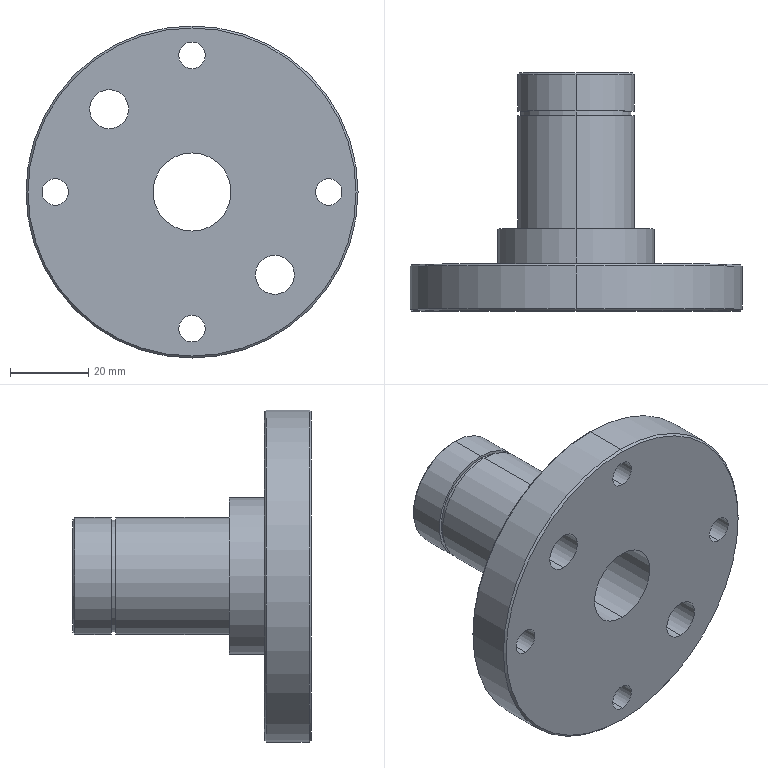Part | SolidWorks | features HoleWzd 2, Chamfer 1, ICE 1, RevCut 1, Revolution 1 | 1 solid | 38 faces | box 85 x 61 x 85 mm | volume 84723 mm3 | cylinder 24 | cone 8 | plane 6 | commonest cylinder face diameters 6.8 x8 10 x4 30 x4 20 x2 28.6 x2 40 x2
STEP:
#1=CARTESIAN_POINT('',(0.,60.5,-10.));
#2=VERTEX_POINT('',#1);
#3=CARTESIAN_POINT('',(0.,60.5,10.));
#4=VERTEX_POINT('',#3);
#5=CARTESIAN_POINT('',(0.,60.5,0.));
#6=DIRECTION('',(0.,1.,0.));
#7=DIRECTION('',(0.,0.,1.));
#8=AXIS2_PLACEMENT_3D('',#5,#6,#7);
#9=CIRCLE('',#8,10.);
#10=EDGE_CURVE('',#2,#4,#9,.T.);
#11=ORIENTED_EDGE('',*,*,#10,.F.);
#12=CARTESIAN_POINT('',(0.,61.,-10.5));
#13=VERTEX_POINT('',#12);
#14=CARTESIAN_POINT('',(0.,60.5,-10.));
#15=DIRECTION('',(0.,0.7071,-0.7071));
#16=VECTOR('',#15,1000.);
#17=LINE('',#14,#16);
#18=EDGE_CURVE('',#2,#13,#17,.T.);
#19=ORIENTED_EDGE('',*,*,#18,.T.);
#20=CARTESIAN_POINT('',(0.,61.,10.5));
#21=VERTEX_POINT('',#20);
#22=CARTESIAN_POINT('',(0.,61.,0.));
#23=DIRECTION('',(0.,-1.,0.));
#24=DIRECTION('',(0.,0.,1.));
#25=AXIS2_PLACEMENT_3D('',#22,#23,#24);
#26=CIRCLE('',#25,10.5);
#27=EDGE_CURVE('',#21,#13,#26,.T.);
#28=ORIENTED_EDGE('',*,*,#27,.F.);
#29=CARTESIAN_POINT('',(0.,60.5,10.));
#30=DIRECTION('',(0.,0.7071,0.7071));
#31=VECTOR('',#30,1000.);
#32=LINE('',#29,#31);
#33=EDGE_CURVE('',#4,#21,#32,.T.);
#34=ORIENTED_EDGE('',*,*,#33,.F.);
#35=EDGE_LOOP('',(#11,#19,#28,#34));
#36=FACE_OUTER_BOUND('',#35,.T.);
#37=CARTESIAN_POINT('',(0.,60.5,0.));
#38=DIRECTION('',(0.,1.,0.));
#39=DIRECTION('',(0.,0.,1.));
#40=AXIS2_PLACEMENT_3D('',#37,#38,#39);
#41=CONICAL_SURFACE('',#40,10.,0.7854);
#42=ADVANCED_FACE('',(#36),#41,.F.);
#43=CARTESIAN_POINT('',(0.,61.,14.5));
#44=VERTEX_POINT('',#43);
#45=CARTESIAN_POINT('',(0.,61.,-14.5));
#46=VERTEX_POINT('',#45);
#47=CARTESIAN_POINT('',(0.,61.,0.));
#48=DIRECTION('',(0.,1.,0.));
#49=DIRECTION('',(0.,0.,1.));
#50=AXIS2_PLACEMENT_3D('',#47,#48,#49);
#51=CIRCLE('',#50,14.5);
#52=EDGE_CURVE('',#44,#46,#51,.T.);
#53=ORIENTED_EDGE('',*,*,#52,.F.);
#54=CARTESIAN_POINT('',(0.,60.5,15.));
#55=VERTEX_POINT('',#54);
#56=CARTESIAN_POINT('',(0.,60.5,15.));
#57=DIRECTION('',(0.,-0.7071,0.7071));
#58=VECTOR('',#57,1000.);
#59=LINE('',#56,#58);
#60=EDGE_CURVE('',#44,#55,#59,.T.);
#61=ORIENTED_EDGE('',*,*,#60,.T.);
#62=CARTESIAN_POINT('',(0.,60.5,-15.));
#63=VERTEX_POINT('',#62);
#64=CARTESIAN_POINT('',(0.,60.5,0.));
#65=DIRECTION('',(0.,-1.,0.));
#66=DIRECTION('',(0.,0.,1.));
#67=AXIS2_PLACEMENT_3D('',#64,#65,#66);
#68=CIRCLE('',#67,15.);
#69=EDGE_CURVE('',#63,#55,#68,.T.);
#70=ORIENTED_EDGE('',*,*,#69,.F.);
#71=CARTESIAN_POINT('',(0.,60.5,-15.));
#72=DIRECTION('',(0.,-0.7071,-0.7071));
#73=VECTOR('',#72,1000.);
#74=LINE('',#71,#73);
#75=EDGE_CURVE('',#46,#63,#74,.T.);
#76=ORIENTED_EDGE('',*,*,#75,.F.);
#77=EDGE_LOOP('',(#53,#61,#70,#76));
#78=FACE_OUTER_BOUND('',#77,.T.);
#79=CARTESIAN_POINT('',(0.,60.5,0.));
#80=DIRECTION('',(0.,-1.,0.));
#81=DIRECTION('',(0.,0.,-1.));
#82=AXIS2_PLACEMENT_3D('',#79,#80,#81);
#83=CONICAL_SURFACE('',#82,15.,0.7854);
#84=ADVANCED_FACE('',(#78),#83,.T.);
#85=CARTESIAN_POINT('',(0.,12.,42.));
#86=VERTEX_POINT('',#85);
#87=CARTESIAN_POINT('',(0.,12.,-42.));
#88=VERTEX_POINT('',#87);
#89=CARTESIAN_POINT('',(0.,12.,0.));
#90=DIRECTION('',(0.,1.,0.));
#91=DIRECTION('',(0.,0.,1.));
#92=AXIS2_PLACEMENT_3D('',#89,#90,#91);
#93=CIRCLE('',#92,42.);
#94=EDGE_CURVE('',#86,#88,#93,.T.);
#95=ORIENTED_EDGE('',*,*,#94,.F.);
#96=CARTESIAN_POINT('',(0.,11.5,42.5));
#97=VERTEX_POINT('',#96);
#98=CARTESIAN_POINT('',(0.,11.5,42.5));
#99=DIRECTION('',(0.,-0.7071,0.7071));
#100=VECTOR('',#99,1000.);
#101=LINE('',#98,#100);
#102=EDGE_CURVE('',#86,#97,#101,.T.);
#103=ORIENTED_EDGE('',*,*,#102,.T.);
#104=CARTESIAN_POINT('',(0.,11.5,-42.5));
#105=VERTEX_POINT('',#104);
#106=CARTESIAN_POINT('',(0.,11.5,0.));
#107=DIRECTION('',(0.,-1.,0.));
#108=DIRECTION('',(0.,0.,1.));
#109=AXIS2_PLACEMENT_3D('',#106,#107,#108);
#110=CIRCLE('',#109,42.5);
#111=EDGE_CURVE('',#105,#97,#110,.T.);
#112=ORIENTED_EDGE('',*,*,#111,.F.);
#113=CARTESIAN_POINT('',(0.,11.5,-42.5));
#114=DIRECTION('',(0.,-0.7071,-0.7071));
#115=VECTOR('',#114,1000.);
#116=LINE('',#113,#115);
#117=EDGE_CURVE('',#88,#105,#116,.T.);
#118=ORIENTED_EDGE('',*,*,#117,.F.);
#119=EDGE_LOOP('',(#95,#103,#112,#118));
#120=FACE_OUTER_BOUND('',#119,.T.);
#121=CARTESIAN_POINT('',(0.,11.5,0.));
#122=DIRECTION('',(0.,-1.,0.));
#123=DIRECTION('',(0.,0.,-1.));
#124=AXIS2_PLACEMENT_3D('',#121,#122,#123);
#125=CONICAL_SURFACE('',#124,42.5,0.7854);
#126=ADVANCED_FACE('',(#120),#125,.T.);
#127=CARTESIAN_POINT('',(0.,0.,-42.));
#128=VERTEX_POINT('',#127);
#129=CARTESIAN_POINT('',(0.,0.,42.));
#130=VERTEX_POINT('',#129);
#131=CARTESIAN_POINT('',(0.,0.,0.));
#132=DIRECTION('',(0.,-1.,0.));
#133=DIRECTION('',(0.,0.,-1.));
#134=AXIS2_PLACEMENT_3D('',#131,#132,#133);
#135=CIRCLE('',#134,42.);
#136=EDGE_CURVE('',#128,#130,#135,.T.);
#137=ORIENTED_EDGE('',*,*,#136,.F.);
#138=CARTESIAN_POINT('',(0.,0.5,-42.5));
#139=VERTEX_POINT('',#138);
#140=CARTESIAN_POINT('',(0.,0.,-42.));
#141=DIRECTION('',(0.,0.7071,-0.7071));
#142=VECTOR('',#141,1000.);
#143=LINE('',#140,#142);
#144=EDGE_CURVE('',#128,#139,#143,.T.);
#145=ORIENTED_EDGE('',*,*,#144,.T.);
#146=CARTESIAN_POINT('',(0.,0.5,42.5));
#147=VERTEX_POINT('',#146);
#148=CARTESIAN_POINT('',(0.,0.5,0.));
#149=DIRECTION('',(0.,1.,0.));
#150=DIRECTION('',(0.,0.,-1.));
#151=AXIS2_PLACEMENT_3D('',#148,#149,#150);
#152=CIRCLE('',#151,42.5);
#153=EDGE_CURVE('',#147,#139,#152,.T.);
#154=ORIENTED_EDGE('',*,*,#153,.F.);
#155=CARTESIAN_POINT('',(0.,0.,42.));
#156=DIRECTION('',(0.,0.7071,0.7071));
#157=VECTOR('',#156,1000.);
#158=LINE('',#155,#157);
#159=EDGE_CURVE('',#130,#147,#158,.T.);
#160=ORIENTED_EDGE('',*,*,#159,.F.);
#161=EDGE_LOOP('',(#137,#145,#154,#160));
#162=FACE_OUTER_BOUND('',#161,.T.);
#163=CARTESIAN_POINT('',(0.,0.,0.));
#164=DIRECTION('',(0.,1.,0.));
#165=DIRECTION('',(0.,0.,1.));
#166=AXIS2_PLACEMENT_3D('',#163,#164,#165);
#167=CONICAL_SURFACE('',#166,42.,0.7854);
#168=ADVANCED_FACE('',(#162),#167,.T.);
#169=CARTESIAN_POINT('',(-21.213,0.,16.213));
#170=VERTEX_POINT('',#169);
#171=CARTESIAN_POINT('',(-21.213,0.,26.213));
#172=VERTEX_POINT('',#171);
#173=CARTESIAN_POINT('',(-21.213,0.,21.213));
#174=DIRECTION('',(0.,1.,0.));
#175=DIRECTION('',(0.,0.,1.));
#176=AXIS2_PLACEMENT_3D('',#173,#174,#175);
#177=CIRCLE('',#176,5.);
#178=EDGE_CURVE('',#170,#172,#177,.T.);
#179=ORIENTED_EDGE('',*,*,#178,.F.);
#180=CARTESIAN_POINT('',(-21.213,12.,16.213));
#181=VERTEX_POINT('',#180);
#182=CARTESIAN_POINT('',(-21.213,12.,16.213));
#183=DIRECTION('',(0.,1.,0.));
#184=VECTOR('',#183,1000.);
#185=LINE('',#182,#184);
#186=EDGE_CURVE('',#170,#181,#185,.T.);
#187=ORIENTED_EDGE('',*,*,#186,.T.);
#188=CARTESIAN_POINT('',(-21.213,12.,26.213));
#189=VERTEX_POINT('',#188);
#190=CARTESIAN_POINT('',(-21.213,12.,21.213));
#191=DIRECTION('',(0.,1.,0.));
#192=DIRECTION('',(0.,0.,1.));
#193=AXIS2_PLACEMENT_3D('',#190,#191,#192);
#194=CIRCLE('',#193,5.);
#195=EDGE_CURVE('',#181,#189,#194,.T.);
#196=ORIENTED_EDGE('',*,*,#195,.T.);
#197=CARTESIAN_POINT('',(-21.213,12.,26.213));
#198=DIRECTION('',(0.,1.,0.));
#199=VECTOR('',#198,1000.);
#200=LINE('',#197,#199);
#201=EDGE_CURVE('',#172,#189,#200,.T.);
#202=ORIENTED_EDGE('',*,*,#201,.F.);
#203=EDGE_LOOP('',(#179,#187,#196,#202));
#204=FACE_OUTER_BOUND('',#203,.T.);
#205=CARTESIAN_POINT('',(-21.213,12.,21.213));
#206=DIRECTION('',(0.,1.,0.));
#207=DIRECTION('',(0.,0.,1.));
#208=AXIS2_PLACEMENT_3D('',#205,#206,#207);
#209=CYLINDRICAL_SURFACE('',#208,5.);
#210=ADVANCED_FACE('',(#204),#209,.F.);
#211=CARTESIAN_POINT('',(21.213,0.,-26.213));
#212=VERTEX_POINT('',#211);
#213=CARTESIAN_POINT('',(21.213,0.,-16.213));
#214=VERTEX_POINT('',#213);
#215=CARTESIAN_POINT('',(21.213,0.,-21.213));
#216=DIRECTION('',(0.,1.,0.));
#217=DIRECTION('',(0.,0.,1.));
#218=AXIS2_PLACEMENT_3D('',#215,#216,#217);
#219=CIRCLE('',#218,5.);
#220=EDGE_CURVE('',#212,#214,#219,.T.);
#221=ORIENTED_EDGE('',*,*,#220,.F.);
#222=CARTESIAN_POINT('',(21.213,12.,-26.213));
#223=VERTEX_POINT('',#222);
#224=CARTESIAN_POINT('',(21.213,12.,-26.213));
#225=DIRECTION('',(0.,1.,0.));
#226=VECTOR('',#225,1000.);
#227=LINE('',#224,#226);
#228=EDGE_CURVE('',#212,#223,#227,.T.);
#229=ORIENTED_EDGE('',*,*,#228,.T.);
#230=CARTESIAN_POINT('',(21.213,12.,-16.213));
#231=VERTEX_POINT('',#230);
#232=CARTESIAN_POINT('',(21.213,12.,-21.213));
#233=DIRECTION('',(0.,1.,0.));
#234=DIRECTION('',(0.,0.,1.));
#235=AXIS2_PLACEMENT_3D('',#232,#233,#234);
#236=CIRCLE('',#235,5.);
#237=EDGE_CURVE('',#223,#231,#236,.T.);
#238=ORIENTED_EDGE('',*,*,#237,.T.);
#239=CARTESIAN_POINT('',(21.213,12.,-16.213));
#240=DIRECTION('',(0.,1.,0.));
#241=VECTOR('',#240,1000.);
#242=LINE('',#239,#241);
#243=EDGE_CURVE('',#214,#231,#242,.T.);
#244=ORIENTED_EDGE('',*,*,#243,.F.);
#245=EDGE_LOOP('',(#221,#229,#238,#244));
#246=FACE_OUTER_BOUND('',#245,.T.);
#247=CARTESIAN_POINT('',(21.213,12.,-21.213));
#248=DIRECTION('',(0.,1.,0.));
#249=DIRECTION('',(0.,0.,1.));
#250=AXIS2_PLACEMENT_3D('',#247,#248,#249);
#251=CYLINDRICAL_SURFACE('',#250,5.);
#252=ADVANCED_FACE('',(#246),#251,.F.);
#253=CARTESIAN_POINT('',(35.,0.,-3.4));
#254=VERTEX_POINT('',#253);
#255=CARTESIAN_POINT('',(35.,0.,3.4));
#256=VERTEX_POINT('',#255);
#257=CARTESIAN_POINT('',(35.,0.,0.));
#258=DIRECTION('',(0.,1.,0.));
#259=DIRECTION('',(0.,0.,1.));
#260=AXIS2_PLACEMENT_3D('',#257,#258,#259);
#261=CIRCLE('',#260,3.4);
#262=EDGE_CURVE('',#254,#256,#261,.T.);
#263=ORIENTED_EDGE('',*,*,#262,.F.);
#264=CARTESIAN_POINT('',(35.,12.,-3.4));
#265=VERTEX_POINT('',#264);
#266=CARTESIAN_POINT('',(35.,12.,-3.4));
#267=DIRECTION('',(0.,1.,0.));
#268=VECTOR('',#267,1000.);
#269=LINE('',#266,#268);
#270=EDGE_CURVE('',#254,#265,#269,.T.);
#271=ORIENTED_EDGE('',*,*,#270,.T.);
#272=CARTESIAN_POINT('',(35.,12.,3.4));
#273=VERTEX_POINT('',#272);
#274=CARTESIAN_POINT('',(35.,12.,0.));
#275=DIRECTION('',(0.,1.,0.));
#276=DIRECTION('',(0.,0.,1.));
#277=AXIS2_PLACEMENT_3D('',#274,#275,#276);
#278=CIRCLE('',#277,3.4);
#279=EDGE_CURVE('',#265,#273,#278,.T.);
#280=ORIENTED_EDGE('',*,*,#279,.T.);
#281=CARTESIAN_POINT('',(35.,12.,3.4));
#282=DIRECTION('',(0.,1.,0.));
#283=VECTOR('',#282,1000.);
#284=LINE('',#281,#283);
#285=EDGE_CURVE('',#256,#273,#284,.T.);
#286=ORIENTED_EDGE('',*,*,#285,.F.);
#287=EDGE_LOOP('',(#263,#271,#280,#286));
#288=FACE_OUTER_BOUND('',#287,.T.);
#289=CARTESIAN_POINT('',(35.,12.,0.));
#290=DIRECTION('',(0.,1.,0.));
#291=DIRECTION('',(0.,0.,1.));
#292=AXIS2_PLACEMENT_3D('',#289,#290,#291);
#293=CYLINDRICAL_SURFACE('',#292,3.4);
#294=ADVANCED_FACE('',(#288),#293,.F.);
#295=CARTESIAN_POINT('',(0.,0.,31.6));
#296=VERTEX_POINT('',#295);
#297=CARTESIAN_POINT('',(0.,0.,38.4));
#298=VERTEX_POINT('',#297);
#299=CARTESIAN_POINT('',(0.,0.,35.));
#300=DIRECTION('',(0.,1.,0.));
#301=DIRECTION('',(0.,0.,1.));
#302=AXIS2_PLACEMENT_3D('',#299,#300,#301);
#303=CIRCLE('',#302,3.4);
#304=EDGE_CURVE('',#296,#298,#303,.T.);
#305=ORIENTED_EDGE('',*,*,#304,.F.);
#306=CARTESIAN_POINT('',(0.,12.,31.6));
#307=VERTEX_POINT('',#306);
#308=CARTESIAN_POINT('',(0.,12.,31.6));
#309=DIRECTION('',(0.,1.,0.));
#310=VECTOR('',#309,1000.);
#311=LINE('',#308,#310);
#312=EDGE_CURVE('',#296,#307,#311,.T.);
#313=ORIENTED_EDGE('',*,*,#312,.T.);
#314=CARTESIAN_POINT('',(0.,12.,38.4));
#315=VERTEX_POINT('',#314);
#316=CARTESIAN_POINT('',(0.,12.,35.));
#317=DIRECTION('',(0.,1.,0.));
#318=DIRECTION('',(0.,0.,1.));
#319=AXIS2_PLACEMENT_3D('',#316,#317,#318);
#320=CIRCLE('',#319,3.4);
#321=EDGE_CURVE('',#307,#315,#320,.T.);
#322=ORIENTED_EDGE('',*,*,#321,.T.);
#323=CARTESIAN_POINT('',(0.,12.,38.4));
#324=DIRECTION('',(0.,1.,0.));
#325=VECTOR('',#324,1000.);
#326=LINE('',#323,#325);
#327=EDGE_CURVE('',#298,#315,#326,.T.);
#328=ORIENTED_EDGE('',*,*,#327,.F.);
#329=EDGE_LOOP('',(#305,#313,#322,#328));
#330=FACE_OUTER_BOUND('',#329,.T.);
#331=CARTESIAN_POINT('',(0.,12.,35.));
#332=DIRECTION('',(0.,1.,0.));
#333=DIRECTION('',(0.,0.,1.));
#334=AXIS2_PLACEMENT_3D('',#331,#332,#333);
#335=CYLINDRICAL_SURFACE('',#334,3.4);
#336=ADVANCED_FACE('',(#330),#335,.F.);
#337=CARTESIAN_POINT('',(-35.,0.,-3.4));
#338=VERTEX_POINT('',#337);
#339=CARTESIAN_POINT('',(-35.,0.,3.4));
#340=VERTEX_POINT('',#339);
#341=CARTESIAN_POINT('',(-35.,0.,0.));
#342=DIRECTION('',(0.,1.,0.));
#343=DIRECTION('',(0.,0.,1.));
#344=AXIS2_PLACEMENT_3D('',#341,#342,#343);
#345=CIRCLE('',#344,3.4);
#346=EDGE_CURVE('',#338,#340,#345,.T.);
#347=ORIENTED_EDGE('',*,*,#346,.F.);
#348=CARTESIAN_POINT('',(-35.,12.,-3.4));
#349=VERTEX_POINT('',#348);
#350=CARTESIAN_POINT('',(-35.,12.,-3.4));
#351=DIRECTION('',(0.,1.,0.));
#352=VECTOR('',#351,1000.);
#353=LINE('',#350,#352);
#354=EDGE_CURVE('',#338,#349,#353,.T.);
#355=ORIENTED_EDGE('',*,*,#354,.T.);
#356=CARTESIAN_POINT('',(-35.,12.,3.4));
#357=VERTEX_POINT('',#356);
#358=CARTESIAN_POINT('',(-35.,12.,0.));
#359=DIRECTION('',(0.,1.,0.));
#360=DIRECTION('',(0.,0.,1.));
#361=AXIS2_PLACEMENT_3D('',#358,#359,#360);
#362=CIRCLE('',#361,3.4);
#363=EDGE_CURVE('',#349,#357,#362,.T.);
#364=ORIENTED_EDGE('',*,*,#363,.T.);
#365=CARTESIAN_POINT('',(-35.,12.,3.4));
#366=DIRECTION('',(0.,1.,0.));
#367=VECTOR('',#366,1000.);
#368=LINE('',#365,#367);
#369=EDGE_CURVE('',#340,#357,#368,.T.);
#370=ORIENTED_EDGE('',*,*,#369,.F.);
#371=EDGE_LOOP('',(#347,#355,#364,#370));
#372=FACE_OUTER_BOUND('',#371,.T.);
#373=CARTESIAN_POINT('',(-35.,12.,0.));
#374=DIRECTION('',(0.,1.,0.));
#375=DIRECTION('',(0.,0.,1.));
#376=AXIS2_PLACEMENT_3D('',#373,#374,#375);
#377=CYLINDRICAL_SURFACE('',#376,3.4);
#378=ADVANCED_FACE('',(#372),#377,.F.);
#379=CARTESIAN_POINT('',(0.,0.,-38.4));
#380=VERTEX_POINT('',#379);
#381=CARTESIAN_POINT('',(0.,0.,-31.6));
#382=VERTEX_POINT('',#381);
#383=CARTESIAN_POINT('',(0.,0.,-35.));
#384=DIRECTION('',(0.,1.,0.));
#385=DIRECTION('',(0.,0.,1.));
#386=AXIS2_PLACEMENT_3D('',#383,#384,#385);
#387=CIRCLE('',#386,3.4);
#388=EDGE_CURVE('',#380,#382,#387,.T.);
#389=ORIENTED_EDGE('',*,*,#388,.F.);
#390=CARTESIAN_POINT('',(0.,12.,-38.4));
#391=VERTEX_POINT('',#390);
#392=CARTESIAN_POINT('',(0.,12.,-38.4));
#393=DIRECTION('',(0.,1.,0.));
#394=VECTOR('',#393,1000.);
#395=LINE('',#392,#394);
#396=EDGE_CURVE('',#380,#391,#395,.T.);
#397=ORIENTED_EDGE('',*,*,#396,.T.);
#398=CARTESIAN_POINT('',(0.,12.,-31.6));
#399=VERTEX_POINT('',#398);
#400=CARTESIAN_POINT('',(0.,12.,-35.));
#401=DIRECTION('',(0.,1.,0.));
#402=DIRECTION('',(0.,0.,1.));
#403=AXIS2_PLACEMENT_3D('',#400,#401,#402);
#404=CIRCLE('',#403,3.4);
#405=EDGE_CURVE('',#391,#399,#404,.T.);
#406=ORIENTED_EDGE('',*,*,#405,.T.);
#407=CARTESIAN_POINT('',(0.,12.,-31.6));
#408=DIRECTION('',(0.,1.,0.));
#409=VECTOR('',#408,1000.);
#410=LINE('',#407,#409);
#411=EDGE_CURVE('',#382,#399,#410,.T.);
#412=ORIENTED_EDGE('',*,*,#411,.F.);
#413=EDGE_LOOP('',(#389,#397,#406,#412));
#414=FACE_OUTER_BOUND('',#413,.T.);
#415=CARTESIAN_POINT('',(0.,12.,-35.));
#416=DIRECTION('',(0.,1.,0.));
#417=DIRECTION('',(0.,0.,1.));
#418=AXIS2_PLACEMENT_3D('',#415,#416,#417);
#419=CYLINDRICAL_SURFACE('',#418,3.4);
#420=ADVANCED_FACE('',(#414),#419,.F.);
#421=CARTESIAN_POINT('',(0.,50.,14.3));
#422=VERTEX_POINT('',#421);
#423=CARTESIAN_POINT('',(0.,50.,-14.3));
#424=VERTEX_POINT('',#423);
#425=CARTESIAN_POINT('',(0.,50.,0.));
#426=DIRECTION('',(0.,1.,0.));
#427=DIRECTION('',(0.,0.,1.));
#428=AXIS2_PLACEMENT_3D('',#425,#426,#427);
#429=CIRCLE('',#428,14.3);
#430=EDGE_CURVE('',#422,#424,#429,.T.);
#431=ORIENTED_EDGE('',*,*,#430,.T.);
#432=CARTESIAN_POINT('',(0.,51.2,-14.3));
#433=VERTEX_POINT('',#432);
#434=CARTESIAN_POINT('',(0.,61.,-14.3));
#435=DIRECTION('',(0.,1.,0.));
#436=VECTOR('',#435,1000.);
#437=LINE('',#434,#436);
#438=EDGE_CURVE('',#424,#433,#437,.T.);
#439=ORIENTED_EDGE('',*,*,#438,.T.);
#440=CARTESIAN_POINT('',(0.,51.2,14.3));
#441=VERTEX_POINT('',#440);
#442=CARTESIAN_POINT('',(0.,51.2,0.));
#443=DIRECTION('',(0.,1.,0.));
#444=DIRECTION('',(0.,0.,1.));
#445=AXIS2_PLACEMENT_3D('',#442,#443,#444);
#446=CIRCLE('',#445,14.3);
#447=EDGE_CURVE('',#441,#433,#446,.T.);
#448=ORIENTED_EDGE('',*,*,#447,.F.);
#449=CARTESIAN_POINT('',(0.,61.,14.3));
#450=DIRECTION('',(0.,1.,0.));
#451=VECTOR('',#450,1000.);
#452=LINE('',#449,#451);
#453=EDGE_CURVE('',#422,#441,#452,.T.);
#454=ORIENTED_EDGE('',*,*,#453,.F.);
#455=EDGE_LOOP('',(#431,#439,#448,#454));
#456=FACE_OUTER_BOUND('',#455,.T.);
#457=CARTESIAN_POINT('',(0.,61.,0.));
#458=DIRECTION('',(0.,1.,0.));
#459=DIRECTION('',(0.,0.,1.));
#460=AXIS2_PLACEMENT_3D('',#457,#458,#459);
#461=CYLINDRICAL_SURFACE('',#460,14.3);
#462=ADVANCED_FACE('',(#456),#461,.T.);
#463=CARTESIAN_POINT('',(0.,0.,-10.));
#464=VERTEX_POINT('',#463);
#465=CARTESIAN_POINT('',(0.,0.,10.));
#466=VERTEX_POINT('',#465);
#467=CARTESIAN_POINT('',(0.,0.,0.));
#468=DIRECTION('',(0.,1.,0.));
#469=DIRECTION('',(0.,0.,1.));
#470=AXIS2_PLACEMENT_3D('',#467,#468,#469);
#471=CIRCLE('',#470,10.);
#472=EDGE_CURVE('',#464,#466,#471,.T.);
#473=ORIENTED_EDGE('',*,*,#472,.F.);
#474=CARTESIAN_POINT('',(0.,0.,-10.));
#475=DIRECTION('',(0.,1.,0.));
#476=VECTOR('',#475,1000.);
#477=LINE('',#474,#476);
#478=EDGE_CURVE('',#464,#2,#477,.T.);
#479=ORIENTED_EDGE('',*,*,#478,.T.);
#480=ORIENTED_EDGE('',*,*,#10,.T.);
#481=CARTESIAN_POINT('',(0.,0.,10.));
#482=DIRECTION('',(0.,1.,0.));
#483=VECTOR('',#482,1000.);
#484=LINE('',#481,#483);
#485=EDGE_CURVE('',#466,#4,#484,.T.);
#486=ORIENTED_EDGE('',*,*,#485,.F.);
#487=EDGE_LOOP('',(#473,#479,#480,#486));
#488=FACE_OUTER_BOUND('',#487,.T.);
#489=CARTESIAN_POINT('',(0.,0.,0.));
#490=DIRECTION('',(0.,1.,0.));
#491=DIRECTION('',(0.,0.,1.));
#492=AXIS2_PLACEMENT_3D('',#489,#490,#491);
#493=CYLINDRICAL_SURFACE('',#492,10.);
#494=ADVANCED_FACE('',(#488),#493,.F.);
#495=CARTESIAN_POINT('',(0.,21.,-20.));
#496=VERTEX_POINT('',#495);
#497=CARTESIAN_POINT('',(0.,21.,20.));
#498=VERTEX_POINT('',#497);
#499=CARTESIAN_POINT('',(0.,21.,0.));
#500=DIRECTION('',(0.,-1.,0.));
#501=DIRECTION('',(0.,0.,-1.));
#502=AXIS2_PLACEMENT_3D('',#499,#500,#501);
#503=CIRCLE('',#502,20.);
#504=EDGE_CURVE('',#496,#498,#503,.T.);
#505=ORIENTED_EDGE('',*,*,#504,.T.);
#506=CARTESIAN_POINT('',(0.,12.,20.));
#507=VERTEX_POINT('',#506);
#508=CARTESIAN_POINT('',(0.,0.,20.));
#509=DIRECTION('',(0.,-1.,0.));
#510=VECTOR('',#509,1000.);
#511=LINE('',#508,#510);
#512=EDGE_CURVE('',#498,#507,#511,.T.);
#513=ORIENTED_EDGE('',*,*,#512,.T.);
#514=CARTESIAN_POINT('',(0.,12.,-20.));
#515=VERTEX_POINT('',#514);
#516=CARTESIAN_POINT('',(0.,12.,0.));
#517=DIRECTION('',(0.,-1.,0.));
#518=DIRECTION('',(0.,0.,-1.));
#519=AXIS2_PLACEMENT_3D('',#516,#517,#518);
#520=CIRCLE('',#519,20.);
#521=EDGE_CURVE('',#515,#507,#520,.T.);
#522=ORIENTED_EDGE('',*,*,#521,.F.);
#523=CARTESIAN_POINT('',(0.,0.,-20.));
#524=DIRECTION('',(0.,-1.,0.));
#525=VECTOR('',#524,1000.);
#526=LINE('',#523,#525);
#527=EDGE_CURVE('',#496,#515,#526,.T.);
#528=ORIENTED_EDGE('',*,*,#527,.F.);
#529=EDGE_LOOP('',(#505,#513,#522,#528));
#530=FACE_OUTER_BOUND('',#529,.T.);
#531=CARTESIAN_POINT('',(0.,0.,0.));
#532=DIRECTION('',(0.,-1.,0.));
#533=DIRECTION('',(0.,0.,-1.));
#534=AXIS2_PLACEMENT_3D('',#531,#532,#533);
#535=CYLINDRICAL_SURFACE('',#534,20.);
#536=ADVANCED_FACE('',(#530),#535,.T.);
#537=ORIENTED_EDGE('',*,*,#111,.T.);
#538=CARTESIAN_POINT('',(0.,0.,42.5));
#539=DIRECTION('',(0.,-1.,0.));
#540=VECTOR('',#539,1000.);
#541=LINE('',#538,#540);
#542=EDGE_CURVE('',#97,#147,#541,.T.);
#543=ORIENTED_EDGE('',*,*,#542,.T.);
#544=ORIENTED_EDGE('',*,*,#153,.T.);
#545=CARTESIAN_POINT('',(0.,0.,-42.5));
#546=DIRECTION('',(0.,-1.,0.));
#547=VECTOR('',#546,1000.);
#548=LINE('',#545,#547);
#549=EDGE_CURVE('',#105,#139,#548,.T.);
#550=ORIENTED_EDGE('',*,*,#549,.F.);
#551=EDGE_LOOP('',(#537,#543,#544,#550));
#552=FACE_OUTER_BOUND('',#551,.T.);
#553=CARTESIAN_POINT('',(0.,0.,0.));
#554=DIRECTION('',(0.,-1.,0.));
#555=DIRECTION('',(0.,0.,-1.));
#556=AXIS2_PLACEMENT_3D('',#553,#554,#555);
#557=CYLINDRICAL_SURFACE('',#556,42.5);
#558=ADVANCED_FACE('',(#552),#557,.T.);
#559=ORIENTED_EDGE('',*,*,#69,.T.);
#560=CARTESIAN_POINT('',(0.,51.2,15.));
#561=VERTEX_POINT('',#560);
#562=CARTESIAN_POINT('',(0.,0.,15.));
#563=DIRECTION('',(0.,-1.,0.));
#564=VECTOR('',#563,1000.);
#565=LINE('',#562,#564);
#566=EDGE_CURVE('',#55,#561,#565,.T.);
#567=ORIENTED_EDGE('',*,*,#566,.T.);
#568=CARTESIAN_POINT('',(0.,51.2,-15.));
#569=VERTEX_POINT('',#568);
#570=CARTESIAN_POINT('',(0.,51.2,0.));
#571=DIRECTION('',(0.,1.,0.));
#572=DIRECTION('',(0.,0.,1.));
#573=AXIS2_PLACEMENT_3D('',#570,#571,#572);
#574=CIRCLE('',#573,15.);
#575=EDGE_CURVE('',#561,#569,#574,.T.);
#576=ORIENTED_EDGE('',*,*,#575,.T.);
#577=CARTESIAN_POINT('',(0.,0.,-15.));
#578=DIRECTION('',(0.,-1.,0.));
#579=VECTOR('',#578,1000.);
#580=LINE('',#577,#579);
#581=EDGE_CURVE('',#63,#569,#580,.T.);
#582=ORIENTED_EDGE('',*,*,#581,.F.);
#583=EDGE_LOOP('',(#559,#567,#576,#582));
#584=FACE_OUTER_BOUND('',#583,.T.);
#585=CARTESIAN_POINT('',(0.,0.,0.));
#586=DIRECTION('',(0.,-1.,0.));
#587=DIRECTION('',(0.,0.,-1.));
#588=AXIS2_PLACEMENT_3D('',#585,#586,#587);
#589=CYLINDRICAL_SURFACE('',#588,15.);
#590=ADVANCED_FACE('',(#584),#589,.T.);
#591=CARTESIAN_POINT('',(0.,50.,15.));
#592=VERTEX_POINT('',#591);
#593=CARTESIAN_POINT('',(0.,50.,-15.));
#594=VERTEX_POINT('',#593);
#595=CARTESIAN_POINT('',(0.,50.,0.));
#596=DIRECTION('',(0.,1.,0.));
#597=DIRECTION('',(0.,0.,1.));
#598=AXIS2_PLACEMENT_3D('',#595,#596,#597);
#599=CIRCLE('',#598,15.);
#600=EDGE_CURVE('',#592,#594,#599,.T.);
#601=ORIENTED_EDGE('',*,*,#600,.F.);
#602=CARTESIAN_POINT('',(0.,21.,15.));
#603=VERTEX_POINT('',#602);
#604=CARTESIAN_POINT('',(0.,0.,15.));
#605=DIRECTION('',(0.,-1.,0.));
#606=VECTOR('',#605,1000.);
#607=LINE('',#604,#606);
#608=EDGE_CURVE('',#592,#603,#607,.T.);
#609=ORIENTED_EDGE('',*,*,#608,.T.);
#610=CARTESIAN_POINT('',(0.,21.,-15.));
#611=VERTEX_POINT('',#610);
#612=CARTESIAN_POINT('',(0.,21.,0.));
#613=DIRECTION('',(0.,-1.,0.));
#614=DIRECTION('',(0.,0.,-1.));
#615=AXIS2_PLACEMENT_3D('',#612,#613,#614);
#616=CIRCLE('',#615,15.);
#617=EDGE_CURVE('',#611,#603,#616,.T.);
#618=ORIENTED_EDGE('',*,*,#617,.F.);
#619=CARTESIAN_POINT('',(0.,0.,-15.));
#620=DIRECTION('',(0.,-1.,0.));
#621=VECTOR('',#620,1000.);
#622=LINE('',#619,#621);
#623=EDGE_CURVE('',#594,#611,#622,.T.);
#624=ORIENTED_EDGE('',*,*,#623,.F.);
#625=EDGE_LOOP('',(#601,#609,#618,#624));
#626=FACE_OUTER_BOUND('',#625,.T.);
#627=CARTESIAN_POINT('',(0.,0.,0.));
#628=DIRECTION('',(0.,-1.,0.));
#629=DIRECTION('',(0.,0.,-1.));
#630=AXIS2_PLACEMENT_3D('',#627,#628,#629);
#631=CYLINDRICAL_SURFACE('',#630,15.);
#632=ADVANCED_FACE('',(#626),#631,.T.);
#633=ORIENTED_EDGE('',*,*,#608,.F.);
#634=CARTESIAN_POINT('',(0.,50.,0.));
#635=DIRECTION('',(0.,1.,0.));
#636=DIRECTION('',(0.,0.,1.));
#637=AXIS2_PLACEMENT_3D('',#634,#635,#636);
#638=CIRCLE('',#637,15.);
#639=EDGE_CURVE('',#594,#592,#638,.T.);
#640=ORIENTED_EDGE('',*,*,#639,.F.);
#641=ORIENTED_EDGE('',*,*,#623,.T.);
#642=CARTESIAN_POINT('',(0.,21.,0.));
#643=DIRECTION('',(0.,-1.,0.));
#644=DIRECTION('',(0.,0.,-1.));
#645=AXIS2_PLACEMENT_3D('',#642,#643,#644);
#646=CIRCLE('',#645,15.);
#647=EDGE_CURVE('',#603,#611,#646,.T.);
#648=ORIENTED_EDGE('',*,*,#647,.F.);
#649=EDGE_LOOP('',(#633,#640,#641,#648));
#650=FACE_OUTER_BOUND('',#649,.T.);
#651=CARTESIAN_POINT('',(0.,0.,0.));
#652=DIRECTION('',(0.,-1.,0.));
#653=DIRECTION('',(0.,0.,-1.));
#654=AXIS2_PLACEMENT_3D('',#651,#652,#653);
#655=CYLINDRICAL_SURFACE('',#654,15.);
#656=ADVANCED_FACE('',(#650),#655,.T.);
#657=ORIENTED_EDGE('',*,*,#566,.F.);
#658=CARTESIAN_POINT('',(0.,60.5,0.));
#659=DIRECTION('',(0.,-1.,0.));
#660=DIRECTION('',(0.,0.,1.));
#661=AXIS2_PLACEMENT_3D('',#658,#659,#660);
#662=CIRCLE('',#661,15.);
#663=EDGE_CURVE('',#55,#63,#662,.T.);
#664=ORIENTED_EDGE('',*,*,#663,.T.);
#665=ORIENTED_EDGE('',*,*,#581,.T.);
#666=CARTESIAN_POINT('',(0.,51.2,0.));
#667=DIRECTION('',(0.,1.,0.));
#668=DIRECTION('',(0.,0.,1.));
#669=AXIS2_PLACEMENT_3D('',#666,#667,#668);
#670=CIRCLE('',#669,15.);
#671=EDGE_CURVE('',#569,#561,#670,.T.);
#672=ORIENTED_EDGE('',*,*,#671,.T.);
#673=EDGE_LOOP('',(#657,#664,#665,#672));
#674=FACE_OUTER_BOUND('',#673,.T.);
#675=CARTESIAN_POINT('',(0.,0.,0.));
#676=DIRECTION('',(0.,-1.,0.));
#677=DIRECTION('',(0.,0.,-1.));
#678=AXIS2_PLACEMENT_3D('',#675,#676,#677);
#679=CYLINDRICAL_SURFACE('',#678,15.);
#680=ADVANCED_FACE('',(#674),#679,.T.);
#681=CARTESIAN_POINT('',(0.,0.,0.));
#682=DIRECTION('',(0.,-1.,0.));
#683=DIRECTION('',(0.,0.,-1.));
#684=AXIS2_PLACEMENT_3D('',#681,#682,#683);
#685=CIRCLE('',#684,42.);
#686=EDGE_CURVE('',#130,#128,#685,.T.);
#687=ORIENTED_EDGE('',*,*,#686,.T.);
#688=ORIENTED_EDGE('',*,*,#136,.T.);
#689=EDGE_LOOP('',(#687,#688));
#690=FACE_OUTER_BOUND('',#689,.T.);
#691=CARTESIAN_POINT('',(-21.213,0.,21.213));
#692=DIRECTION('',(0.,1.,0.));
#693=DIRECTION('',(0.,0.,1.));
#694=AXIS2_PLACEMENT_3D('',#691,#692,#693);
#695=CIRCLE('',#694,5.);
#696=EDGE_CURVE('',#172,#170,#695,.T.);
#697=ORIENTED_EDGE('',*,*,#696,.T.);
#698=ORIENTED_EDGE('',*,*,#178,.T.);
#699=EDGE_LOOP('',(#697,#698));
#700=FACE_BOUND('',#699,.T.);
#701=CARTESIAN_POINT('',(21.213,0.,-21.213));
#702=DIRECTION('',(0.,1.,0.));
#703=DIRECTION('',(0.,0.,1.));
#704=AXIS2_PLACEMENT_3D('',#701,#702,#703);
#705=CIRCLE('',#704,5.);
#706=EDGE_CURVE('',#214,#212,#705,.T.);
#707=ORIENTED_EDGE('',*,*,#706,.T.);
#708=ORIENTED_EDGE('',*,*,#220,.T.);
#709=EDGE_LOOP('',(#707,#708));
#710=FACE_BOUND('',#709,.T.);
#711=CARTESIAN_POINT('',(35.,0.,0.));
#712=DIRECTION('',(0.,1.,0.));
#713=DIRECTION('',(0.,0.,1.));
#714=AXIS2_PLACEMENT_3D('',#711,#712,#713);
#715=CIRCLE('',#714,3.4);
#716=EDGE_CURVE('',#256,#254,#715,.T.);
#717=ORIENTED_EDGE('',*,*,#716,.T.);
#718=ORIENTED_EDGE('',*,*,#262,.T.);
#719=EDGE_LOOP('',(#717,#718));
#720=FACE_BOUND('',#719,.T.);
#721=CARTESIAN_POINT('',(0.,0.,35.));
#722=DIRECTION('',(0.,1.,0.));
#723=DIRECTION('',(0.,0.,1.));
#724=AXIS2_PLACEMENT_3D('',#721,#722,#723);
#725=CIRCLE('',#724,3.4);
#726=EDGE_CURVE('',#298,#296,#725,.T.);
#727=ORIENTED_EDGE('',*,*,#726,.T.);
#728=ORIENTED_EDGE('',*,*,#304,.T.);
#729=EDGE_LOOP('',(#727,#728));
#730=FACE_BOUND('',#729,.T.);
#731=CARTESIAN_POINT('',(-35.,0.,0.));
#732=DIRECTION('',(0.,1.,0.));
#733=DIRECTION('',(0.,0.,1.));
#734=AXIS2_PLACEMENT_3D('',#731,#732,#733);
#735=CIRCLE('',#734,3.4);
#736=EDGE_CURVE('',#340,#338,#735,.T.);
#737=ORIENTED_EDGE('',*,*,#736,.T.);
#738=ORIENTED_EDGE('',*,*,#346,.T.);
#739=EDGE_LOOP('',(#737,#738));
#740=FACE_BOUND('',#739,.T.);
#741=CARTESIAN_POINT('',(0.,0.,-35.));
#742=DIRECTION('',(0.,1.,0.));
#743=DIRECTION('',(0.,0.,1.));
#744=AXIS2_PLACEMENT_3D('',#741,#742,#743);
#745=CIRCLE('',#744,3.4);
#746=EDGE_CURVE('',#382,#380,#745,.T.);
#747=ORIENTED_EDGE('',*,*,#746,.T.);
#748=ORIENTED_EDGE('',*,*,#388,.T.);
#749=EDGE_LOOP('',(#747,#748));
#750=FACE_BOUND('',#749,.T.);
#751=CARTESIAN_POINT('',(0.,0.,0.));
#752=DIRECTION('',(0.,1.,0.));
#753=DIRECTION('',(0.,0.,1.));
#754=AXIS2_PLACEMENT_3D('',#751,#752,#753);
#755=CIRCLE('',#754,10.);
#756=EDGE_CURVE('',#466,#464,#755,.T.);
#757=ORIENTED_EDGE('',*,*,#756,.T.);
#758=ORIENTED_EDGE('',*,*,#472,.T.);
#759=EDGE_LOOP('',(#757,#758));
#760=FACE_BOUND('',#759,.T.);
#761=CARTESIAN_POINT('',(0.,0.,0.));
#762=DIRECTION('',(0.,-1.,0.));
#763=DIRECTION('',(0.,0.,-1.));
#764=AXIS2_PLACEMENT_3D('',#761,#762,#763);
#765=PLANE('',#764);
#766=ADVANCED_FACE('',(#690,#700,#710,#720,#730,#740,#750,#760),#765,.T.);
#767=ORIENTED_EDGE('',*,*,#542,.F.);
#768=CARTESIAN_POINT('',(0.,11.5,0.));
#769=DIRECTION('',(0.,-1.,0.));
#770=DIRECTION('',(0.,0.,1.));
#771=AXIS2_PLACEMENT_3D('',#768,#769,#770);
#772=CIRCLE('',#771,42.5);
#773=EDGE_CURVE('',#97,#105,#772,.T.);
#774=ORIENTED_EDGE('',*,*,#773,.T.);
#775=ORIENTED_EDGE('',*,*,#549,.T.);
#776=CARTESIAN_POINT('',(0.,0.5,0.));
#777=DIRECTION('',(0.,1.,0.));
#778=DIRECTION('',(0.,0.,-1.));
#779=AXIS2_PLACEMENT_3D('',#776,#777,#778);
#780=CIRCLE('',#779,42.5);
#781=EDGE_CURVE('',#139,#147,#780,.T.);
#782=ORIENTED_EDGE('',*,*,#781,.T.);
#783=EDGE_LOOP('',(#767,#774,#775,#782));
#784=FACE_OUTER_BOUND('',#783,.T.);
#785=CARTESIAN_POINT('',(0.,0.,0.));
#786=DIRECTION('',(0.,-1.,0.));
#787=DIRECTION('',(0.,0.,-1.));
#788=AXIS2_PLACEMENT_3D('',#785,#786,#787);
#789=CYLINDRICAL_SURFACE('',#788,42.5);
#790=ADVANCED_FACE('',(#784),#789,.T.);
#791=CARTESIAN_POINT('',(0.,12.,0.));
#792=DIRECTION('',(0.,1.,0.));
#793=DIRECTION('',(0.,0.,1.));
#794=AXIS2_PLACEMENT_3D('',#791,#792,#793);
#795=CIRCLE('',#794,42.);
#796=EDGE_CURVE('',#88,#86,#795,.T.);
#797=ORIENTED_EDGE('',*,*,#796,.T.);
#798=ORIENTED_EDGE('',*,*,#94,.T.);
#799=EDGE_LOOP('',(#797,#798));
#800=FACE_OUTER_BOUND('',#799,.T.);
#801=CARTESIAN_POINT('',(-21.213,12.,21.213));
#802=DIRECTION('',(0.,1.,0.));
#803=DIRECTION('',(0.,0.,1.));
#804=AXIS2_PLACEMENT_3D('',#801,#802,#803);
#805=CIRCLE('',#804,5.);
#806=EDGE_CURVE('',#189,#181,#805,.T.);
#807=ORIENTED_EDGE('',*,*,#806,.F.);
#808=ORIENTED_EDGE('',*,*,#195,.F.);
#809=EDGE_LOOP('',(#807,#808));
#810=FACE_BOUND('',#809,.T.);
#811=CARTESIAN_POINT('',(21.213,12.,-21.213));
#812=DIRECTION('',(0.,1.,0.));
#813=DIRECTION('',(0.,0.,1.));
#814=AXIS2_PLACEMENT_3D('',#811,#812,#813);
#815=CIRCLE('',#814,5.);
#816=EDGE_CURVE('',#231,#223,#815,.T.);
#817=ORIENTED_EDGE('',*,*,#816,.F.);
#818=ORIENTED_EDGE('',*,*,#237,.F.);
#819=EDGE_LOOP('',(#817,#818));
#820=FACE_BOUND('',#819,.T.);
#821=CARTESIAN_POINT('',(35.,12.,0.));
#822=DIRECTION('',(0.,1.,0.));
#823=DIRECTION('',(0.,0.,1.));
#824=AXIS2_PLACEMENT_3D('',#821,#822,#823);
#825=CIRCLE('',#824,3.4);
#826=EDGE_CURVE('',#273,#265,#825,.T.);
#827=ORIENTED_EDGE('',*,*,#826,.F.);
#828=ORIENTED_EDGE('',*,*,#279,.F.);
#829=EDGE_LOOP('',(#827,#828));
#830=FACE_BOUND('',#829,.T.);
#831=CARTESIAN_POINT('',(0.,12.,35.));
#832=DIRECTION('',(0.,1.,0.));
#833=DIRECTION('',(0.,0.,1.));
#834=AXIS2_PLACEMENT_3D('',#831,#832,#833);
#835=CIRCLE('',#834,3.4);
#836=EDGE_CURVE('',#315,#307,#835,.T.);
#837=ORIENTED_EDGE('',*,*,#836,.F.);
#838=ORIENTED_EDGE('',*,*,#321,.F.);
#839=EDGE_LOOP('',(#837,#838));
#840=FACE_BOUND('',#839,.T.);
#841=CARTESIAN_POINT('',(-35.,12.,0.));
#842=DIRECTION('',(0.,1.,0.));
#843=DIRECTION('',(0.,0.,1.));
#844=AXIS2_PLACEMENT_3D('',#841,#842,#843);
#845=CIRCLE('',#844,3.4);
#846=EDGE_CURVE('',#357,#349,#845,.T.);
#847=ORIENTED_EDGE('',*,*,#846,.F.);
#848=ORIENTED_EDGE('',*,*,#363,.F.);
#849=EDGE_LOOP('',(#847,#848));
#850=FACE_BOUND('',#849,.T.);
#851=CARTESIAN_POINT('',(0.,12.,-35.));
#852=DIRECTION('',(0.,1.,0.));
#853=DIRECTION('',(0.,0.,1.));
#854=AXIS2_PLACEMENT_3D('',#851,#852,#853);
#855=CIRCLE('',#854,3.4);
#856=EDGE_CURVE('',#399,#391,#855,.T.);
#857=ORIENTED_EDGE('',*,*,#856,.F.);
#858=ORIENTED_EDGE('',*,*,#405,.F.);
#859=EDGE_LOOP('',(#857,#858));
#860=FACE_BOUND('',#859,.T.);
#861=ORIENTED_EDGE('',*,*,#521,.T.);
#862=CARTESIAN_POINT('',(0.,12.,0.));
#863=DIRECTION('',(0.,-1.,0.));
#864=DIRECTION('',(0.,0.,-1.));
#865=AXIS2_PLACEMENT_3D('',#862,#863,#864);
#866=CIRCLE('',#865,20.);
#867=EDGE_CURVE('',#507,#515,#866,.T.);
#868=ORIENTED_EDGE('',*,*,#867,.T.);
#869=EDGE_LOOP('',(#861,#868));
#870=FACE_BOUND('',#869,.T.);
#871=CARTESIAN_POINT('',(42.5,12.,0.));
#872=DIRECTION('',(0.,1.,0.));
#873=DIRECTION('',(0.,0.,1.));
#874=AXIS2_PLACEMENT_3D('',#871,#872,#873);
#875=PLANE('',#874);
#876=ADVANCED_FACE('',(#800,#810,#820,#830,#840,#850,#860,#870),#875,.T.);
#877=ORIENTED_EDGE('',*,*,#512,.F.);
#878=CARTESIAN_POINT('',(0.,21.,0.));
#879=DIRECTION('',(0.,-1.,0.));
#880=DIRECTION('',(0.,0.,-1.));
#881=AXIS2_PLACEMENT_3D('',#878,#879,#880);
#882=CIRCLE('',#881,20.);
#883=EDGE_CURVE('',#498,#496,#882,.T.);
#884=ORIENTED_EDGE('',*,*,#883,.T.);
#885=ORIENTED_EDGE('',*,*,#527,.T.);
#886=ORIENTED_EDGE('',*,*,#867,.F.);
#887=EDGE_LOOP('',(#877,#884,#885,#886));
#888=FACE_OUTER_BOUND('',#887,.T.);
#889=CARTESIAN_POINT('',(0.,0.,0.));
#890=DIRECTION('',(0.,-1.,0.));
#891=DIRECTION('',(0.,0.,-1.));
#892=AXIS2_PLACEMENT_3D('',#889,#890,#891);
#893=CYLINDRICAL_SURFACE('',#892,20.);
#894=ADVANCED_FACE('',(#888),#893,.T.);
#895=ORIENTED_EDGE('',*,*,#617,.T.);
#896=ORIENTED_EDGE('',*,*,#647,.T.);
#897=EDGE_LOOP('',(#895,#896));
#898=FACE_BOUND('',#897,.T.);
#899=ORIENTED_EDGE('',*,*,#504,.F.);
#900=ORIENTED_EDGE('',*,*,#883,.F.);
#901=EDGE_LOOP('',(#899,#900));
#902=FACE_OUTER_BOUND('',#901,.T.);
#903=CARTESIAN_POINT('',(20.,21.,0.));
#904=DIRECTION('',(0.,1.,0.));
#905=DIRECTION('',(0.,0.,1.));
#906=AXIS2_PLACEMENT_3D('',#903,#904,#905);
#907=PLANE('',#906);
#908=ADVANCED_FACE('',(#898,#902),#907,.T.);
#909=CARTESIAN_POINT('',(0.,61.,0.));
#910=DIRECTION('',(0.,1.,0.));
#911=DIRECTION('',(0.,0.,1.));
#912=AXIS2_PLACEMENT_3D('',#909,#910,#911);
#913=CIRCLE('',#912,14.5);
#914=EDGE_CURVE('',#46,#44,#913,.T.);
#915=ORIENTED_EDGE('',*,*,#914,.T.);
#916=ORIENTED_EDGE('',*,*,#52,.T.);
#917=EDGE_LOOP('',(#915,#916));
#918=FACE_OUTER_BOUND('',#917,.T.);
#919=ORIENTED_EDGE('',*,*,#27,.T.);
#920=CARTESIAN_POINT('',(0.,61.,0.));
#921=DIRECTION('',(0.,-1.,0.));
#922=DIRECTION('',(0.,0.,1.));
#923=AXIS2_PLACEMENT_3D('',#920,#921,#922);
#924=CIRCLE('',#923,10.5);
#925=EDGE_CURVE('',#13,#21,#924,.T.);
#926=ORIENTED_EDGE('',*,*,#925,.T.);
#927=EDGE_LOOP('',(#919,#926));
#928=FACE_BOUND('',#927,.T.);
#929=CARTESIAN_POINT('',(15.,61.,0.));
#930=DIRECTION('',(0.,1.,0.));
#931=DIRECTION('',(0.,0.,1.));
#932=AXIS2_PLACEMENT_3D('',#929,#930,#931);
#933=PLANE('',#932);
#934=ADVANCED_FACE('',(#918,#928),#933,.T.);
#935=ORIENTED_EDGE('',*,*,#478,.F.);
#936=ORIENTED_EDGE('',*,*,#756,.F.);
#937=ORIENTED_EDGE('',*,*,#485,.T.);
#938=CARTESIAN_POINT('',(0.,60.5,0.));
#939=DIRECTION('',(0.,1.,0.));
#940=DIRECTION('',(0.,0.,1.));
#941=AXIS2_PLACEMENT_3D('',#938,#939,#940);
#942=CIRCLE('',#941,10.);
#943=EDGE_CURVE('',#4,#2,#942,.T.);
#944=ORIENTED_EDGE('',*,*,#943,.T.);
#945=EDGE_LOOP('',(#935,#936,#937,#944));
#946=FACE_OUTER_BOUND('',#945,.T.);
#947=CARTESIAN_POINT('',(0.,0.,0.));
#948=DIRECTION('',(0.,1.,0.));
#949=DIRECTION('',(0.,0.,1.));
#950=AXIS2_PLACEMENT_3D('',#947,#948,#949);
#951=CYLINDRICAL_SURFACE('',#950,10.);
#952=ADVANCED_FACE('',(#946),#951,.F.);
#953=ORIENTED_EDGE('',*,*,#639,.T.);
#954=ORIENTED_EDGE('',*,*,#600,.T.);
#955=EDGE_LOOP('',(#953,#954));
#956=FACE_OUTER_BOUND('',#955,.T.);
#957=ORIENTED_EDGE('',*,*,#430,.F.);
#958=CARTESIAN_POINT('',(0.,50.,0.));
#959=DIRECTION('',(0.,1.,0.));
#960=DIRECTION('',(0.,0.,1.));
#961=AXIS2_PLACEMENT_3D('',#958,#959,#960);
#962=CIRCLE('',#961,14.3);
#963=EDGE_CURVE('',#424,#422,#962,.T.);
#964=ORIENTED_EDGE('',*,*,#963,.F.);
#965=EDGE_LOOP('',(#957,#964));
#966=FACE_BOUND('',#965,.T.);
#967=CARTESIAN_POINT('',(15.,50.,0.));
#968=DIRECTION('',(0.,1.,0.));
#969=DIRECTION('',(0.,0.,1.));
#970=AXIS2_PLACEMENT_3D('',#967,#968,#969);
#971=PLANE('',#970);
#972=ADVANCED_FACE('',(#956,#966),#971,.T.);
#973=ORIENTED_EDGE('',*,*,#438,.F.);
#974=ORIENTED_EDGE('',*,*,#963,.T.);
#975=ORIENTED_EDGE('',*,*,#453,.T.);
#976=CARTESIAN_POINT('',(0.,51.2,0.));
#977=DIRECTION('',(0.,1.,0.));
#978=DIRECTION('',(0.,0.,1.));
#979=AXIS2_PLACEMENT_3D('',#976,#977,#978);
#980=CIRCLE('',#979,14.3);
#981=EDGE_CURVE('',#433,#441,#980,.T.);
#982=ORIENTED_EDGE('',*,*,#981,.F.);
#983=EDGE_LOOP('',(#973,#974,#975,#982));
#984=FACE_OUTER_BOUND('',#983,.T.);
#985=CARTESIAN_POINT('',(0.,61.,0.));
#986=DIRECTION('',(0.,1.,0.));
#987=DIRECTION('',(0.,0.,1.));
#988=AXIS2_PLACEMENT_3D('',#985,#986,#987);
#989=CYLINDRICAL_SURFACE('',#988,14.3);
#990=ADVANCED_FACE('',(#984),#989,.T.);
#991=ORIENTED_EDGE('',*,*,#447,.T.);
#992=ORIENTED_EDGE('',*,*,#981,.T.);
#993=EDGE_LOOP('',(#991,#992));
#994=FACE_BOUND('',#993,.T.);
#995=ORIENTED_EDGE('',*,*,#671,.F.);
#996=ORIENTED_EDGE('',*,*,#575,.F.);
#997=EDGE_LOOP('',(#995,#996));
#998=FACE_OUTER_BOUND('',#997,.T.);
#999=CARTESIAN_POINT('',(15.,51.2,0.));
#1000=DIRECTION('',(0.,-1.,0.));
#1001=DIRECTION('',(0.,0.,-1.));
#1002=AXIS2_PLACEMENT_3D('',#999,#1000,#1001);
#1003=PLANE('',#1002);
#1004=ADVANCED_FACE('',(#994,#998),#1003,.T.);
#1005=ORIENTED_EDGE('',*,*,#396,.F.);
#1006=ORIENTED_EDGE('',*,*,#746,.F.);
#1007=ORIENTED_EDGE('',*,*,#411,.T.);
#1008=ORIENTED_EDGE('',*,*,#856,.T.);
#1009=EDGE_LOOP('',(#1005,#1006,#1007,#1008));
#1010=FACE_OUTER_BOUND('',#1009,.T.);
#1011=CARTESIAN_POINT('',(0.,12.,-35.));
#1012=DIRECTION('',(0.,1.,0.));
#1013=DIRECTION('',(0.,0.,1.));
#1014=AXIS2_PLACEMENT_3D('',#1011,#1012,#1013);
#1015=CYLINDRICAL_SURFACE('',#1014,3.4);
#1016=ADVANCED_FACE('',(#1010),#1015,.F.);
#1017=ORIENTED_EDGE('',*,*,#354,.F.);
#1018=ORIENTED_EDGE('',*,*,#736,.F.);
#1019=ORIENTED_EDGE('',*,*,#369,.T.);
#1020=ORIENTED_EDGE('',*,*,#846,.T.);
#1021=EDGE_LOOP('',(#1017,#1018,#1019,#1020));
#1022=FACE_OUTER_BOUND('',#1021,.T.);
#1023=CARTESIAN_POINT('',(-35.,12.,0.));
#1024=DIRECTION('',(0.,1.,0.));
#1025=DIRECTION('',(0.,0.,1.));
#1026=AXIS2_PLACEMENT_3D('',#1023,#1024,#1025);
#1027=CYLINDRICAL_SURFACE('',#1026,3.4);
#1028=ADVANCED_FACE('',(#1022),#1027,.F.);
#1029=ORIENTED_EDGE('',*,*,#312,.F.);
#1030=ORIENTED_EDGE('',*,*,#726,.F.);
#1031=ORIENTED_EDGE('',*,*,#327,.T.);
#1032=ORIENTED_EDGE('',*,*,#836,.T.);
#1033=EDGE_LOOP('',(#1029,#1030,#1031,#1032));
#1034=FACE_OUTER_BOUND('',#1033,.T.);
#1035=CARTESIAN_POINT('',(0.,12.,35.));
#1036=DIRECTION('',(0.,1.,0.));
#1037=DIRECTION('',(0.,0.,1.));
#1038=AXIS2_PLACEMENT_3D('',#1035,#1036,#1037);
#1039=CYLINDRICAL_SURFACE('',#1038,3.4);
#1040=ADVANCED_FACE('',(#1034),#1039,.F.);
#1041=ORIENTED_EDGE('',*,*,#270,.F.);
#1042=ORIENTED_EDGE('',*,*,#716,.F.);
#1043=ORIENTED_EDGE('',*,*,#285,.T.);
#1044=ORIENTED_EDGE('',*,*,#826,.T.);
#1045=EDGE_LOOP('',(#1041,#1042,#1043,#1044));
#1046=FACE_OUTER_BOUND('',#1045,.T.);
#1047=CARTESIAN_POINT('',(35.,12.,0.));
#1048=DIRECTION('',(0.,1.,0.));
#1049=DIRECTION('',(0.,0.,1.));
#1050=AXIS2_PLACEMENT_3D('',#1047,#1048,#1049);
#1051=CYLINDRICAL_SURFACE('',#1050,3.4);
#1052=ADVANCED_FACE('',(#1046),#1051,.F.);
#1053=ORIENTED_EDGE('',*,*,#228,.F.);
#1054=ORIENTED_EDGE('',*,*,#706,.F.);
#1055=ORIENTED_EDGE('',*,*,#243,.T.);
#1056=ORIENTED_EDGE('',*,*,#816,.T.);
#1057=EDGE_LOOP('',(#1053,#1054,#1055,#1056));
#1058=FACE_OUTER_BOUND('',#1057,.T.);
#1059=CARTESIAN_POINT('',(21.213,12.,-21.213));
#1060=DIRECTION('',(0.,1.,0.));
#1061=DIRECTION('',(0.,0.,1.));
#1062=AXIS2_PLACEMENT_3D('',#1059,#1060,#1061);
#1063=CYLINDRICAL_SURFACE('',#1062,5.);
#1064=ADVANCED_FACE('',(#1058),#1063,.F.);
#1065=ORIENTED_EDGE('',*,*,#186,.F.);
#1066=ORIENTED_EDGE('',*,*,#696,.F.);
#1067=ORIENTED_EDGE('',*,*,#201,.T.);
#1068=ORIENTED_EDGE('',*,*,#806,.T.);
#1069=EDGE_LOOP('',(#1065,#1066,#1067,#1068));
#1070=FACE_OUTER_BOUND('',#1069,.T.);
#1071=CARTESIAN_POINT('',(-21.213,12.,21.213));
#1072=DIRECTION('',(0.,1.,0.));
#1073=DIRECTION('',(0.,0.,1.));
#1074=AXIS2_PLACEMENT_3D('',#1071,#1072,#1073);
#1075=CYLINDRICAL_SURFACE('',#1074,5.);
#1076=ADVANCED_FACE('',(#1070),#1075,.F.);
#1077=ORIENTED_EDGE('',*,*,#144,.F.);
#1078=ORIENTED_EDGE('',*,*,#686,.F.);
#1079=ORIENTED_EDGE('',*,*,#159,.T.);
#1080=ORIENTED_EDGE('',*,*,#781,.F.);
#1081=EDGE_LOOP('',(#1077,#1078,#1079,#1080));
#1082=FACE_OUTER_BOUND('',#1081,.T.);
#1083=CARTESIAN_POINT('',(0.,0.,0.));
#1084=DIRECTION('',(0.,1.,0.));
#1085=DIRECTION('',(0.,0.,1.));
#1086=AXIS2_PLACEMENT_3D('',#1083,#1084,#1085);
#1087=CONICAL_SURFACE('',#1086,42.,0.7854);
#1088=ADVANCED_FACE('',(#1082),#1087,.T.);
#1089=ORIENTED_EDGE('',*,*,#102,.F.);
#1090=ORIENTED_EDGE('',*,*,#796,.F.);
#1091=ORIENTED_EDGE('',*,*,#117,.T.);
#1092=ORIENTED_EDGE('',*,*,#773,.F.);
#1093=EDGE_LOOP('',(#1089,#1090,#1091,#1092));
#1094=FACE_OUTER_BOUND('',#1093,.T.);
#1095=CARTESIAN_POINT('',(0.,11.5,0.));
#1096=DIRECTION('',(0.,-1.,0.));
#1097=DIRECTION('',(0.,0.,-1.));
#1098=AXIS2_PLACEMENT_3D('',#1095,#1096,#1097);
#1099=CONICAL_SURFACE('',#1098,42.5,0.7854);
#1100=ADVANCED_FACE('',(#1094),#1099,.T.);
#1101=ORIENTED_EDGE('',*,*,#60,.F.);
#1102=ORIENTED_EDGE('',*,*,#914,.F.);
#1103=ORIENTED_EDGE('',*,*,#75,.T.);
#1104=ORIENTED_EDGE('',*,*,#663,.F.);
#1105=EDGE_LOOP('',(#1101,#1102,#1103,#1104));
#1106=FACE_OUTER_BOUND('',#1105,.T.);
#1107=CARTESIAN_POINT('',(0.,60.5,0.));
#1108=DIRECTION('',(0.,-1.,0.));
#1109=DIRECTION('',(0.,0.,-1.));
#1110=AXIS2_PLACEMENT_3D('',#1107,#1108,#1109);
#1111=CONICAL_SURFACE('',#1110,15.,0.7854);
#1112=ADVANCED_FACE('',(#1106),#1111,.T.);
#1113=ORIENTED_EDGE('',*,*,#18,.F.);
#1114=ORIENTED_EDGE('',*,*,#943,.F.);
#1115=ORIENTED_EDGE('',*,*,#33,.T.);
#1116=ORIENTED_EDGE('',*,*,#925,.F.);
#1117=EDGE_LOOP('',(#1113,#1114,#1115,#1116));
#1118=FACE_OUTER_BOUND('',#1117,.T.);
#1119=CARTESIAN_POINT('',(0.,60.5,0.));
#1120=DIRECTION('',(0.,1.,0.));
#1121=DIRECTION('',(0.,0.,1.));
#1122=AXIS2_PLACEMENT_3D('',#1119,#1120,#1121);
#1123=CONICAL_SURFACE('',#1122,10.,0.7854);
#1124=ADVANCED_FACE('',(#1118),#1123,.F.);
#1125=CLOSED_SHELL('',(#42,#84,#126,#168,#210,#252,#294,#336,#378,#420,#462,#494,#536,#558,#590,#632,#656,#680,#766,#790,#876,#894,#908,#934,#952,#972,#990,#1004,#1016,#1028,#1040,#1052,#1064,#1076,#1088,#1100,#1112,#1124));
#1126=MANIFOLD_SOLID_BREP('',#1125);
#1127=CARTESIAN_POINT('',(0.,0.,0.));
#1128=DIRECTION('',(0.,0.,1.));
#1129=DIRECTION('',(1.,0.,0.));
#1130=AXIS2_PLACEMENT_3D('',#1127,#1128,#1129);
#1131=(LENGTH_UNIT()NAMED_UNIT(*)SI_UNIT(.MILLI.,.METRE.));
#1132=UNCERTAINTY_MEASURE_WITH_UNIT(LENGTH_MEASURE(0.00001),#1131,'','');
#1133=(NAMED_UNIT(*)PLANE_ANGLE_UNIT()SI_UNIT($,.RADIAN.));
#1134=(NAMED_UNIT(*)SI_UNIT($,.STERADIAN.)SOLID_ANGLE_UNIT());
#1135=(GEOMETRIC_REPRESENTATION_CONTEXT(3)GLOBAL_UNCERTAINTY_ASSIGNED_CONTEXT((#1132))GLOBAL_UNIT_ASSIGNED_CONTEXT((#1131,#1133,#1134))REPRESENTATION_CONTEXT('',''));
#1136=ADVANCED_BREP_SHAPE_REPRESENTATION('',(#1126,#1130),#1135);